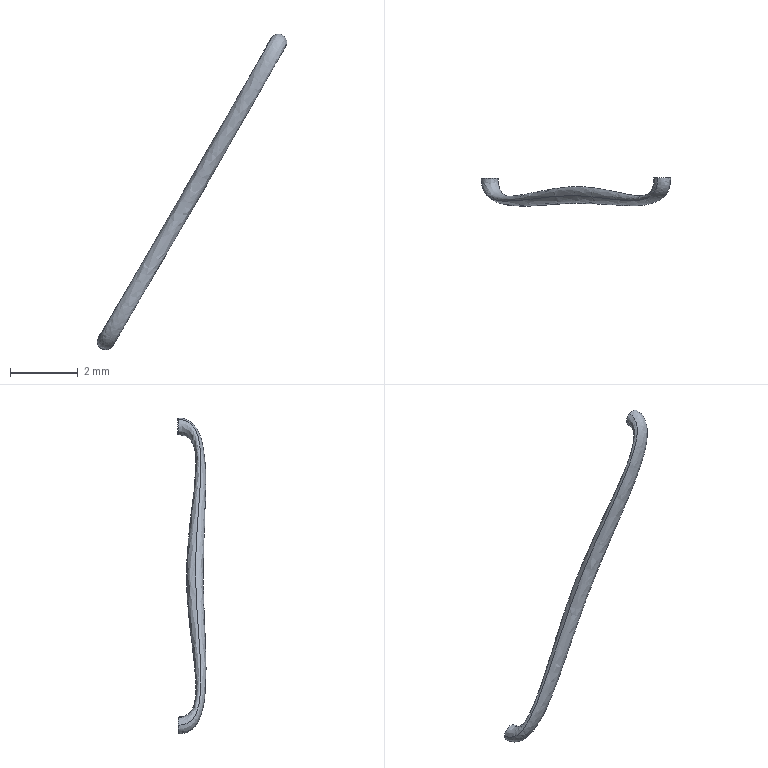Part | SolidWorks | features BaseBody 1 | 1 solid | 4 faces | box 5.609 x 0.83 x 9.35 mm | volume 1.655 mm3 | plane 2 | spline 2
STEP:
#1=CARTESIAN_POINT('',(329.531,392.452,108.323));
#2=VERTEX_POINT('',#1);
#3=CARTESIAN_POINT('',(329.032,392.452,108.347));
#4=VERTEX_POINT('',#3);
#5=CARTESIAN_POINT('',(329.531,392.452,108.323));
#6=CARTESIAN_POINT('',(329.531,392.452,108.316));
#7=CARTESIAN_POINT('',(329.53,392.452,108.303));
#8=CARTESIAN_POINT('',(329.526,392.452,108.283));
#9=CARTESIAN_POINT('',(329.521,392.452,108.263));
#10=CARTESIAN_POINT('',(329.5,392.452,108.201));
#11=CARTESIAN_POINT('',(329.445,392.452,108.134));
#12=CARTESIAN_POINT('',(329.351,392.452,108.091));
#13=CARTESIAN_POINT('',(329.263,392.452,108.08));
#14=CARTESIAN_POINT('',(329.17,392.452,108.104));
#15=CARTESIAN_POINT('',(329.092,392.452,108.163));
#16=CARTESIAN_POINT('',(329.041,392.452,108.246));
#17=CARTESIAN_POINT('',(329.03,392.452,108.314));
#18=CARTESIAN_POINT('',(329.032,392.452,108.347));
#19=B_SPLINE_CURVE_WITH_KNOTS('',3,(#5,#6,#7,#8,#9,#10,#11,#12,#13,#14,#15,#16,#17,#18),.UNSPECIFIED.,.F.,.F.,(4,1,1,1,1,1,1,1,1,1,1,4),(0.,0.025,0.05,0.075,0.1,0.3,0.4,0.5,0.625,0.75,0.875,1.),.UNSPECIFIED.);
#20=EDGE_CURVE('',#2,#4,#19,.T.);
#21=ORIENTED_EDGE('',*,*,#20,.T.);
#22=CARTESIAN_POINT('',(329.032,392.452,108.347));
#23=CARTESIAN_POINT('',(329.034,392.452,108.381));
#24=CARTESIAN_POINT('',(329.051,392.452,108.447));
#25=CARTESIAN_POINT('',(329.11,392.452,108.525));
#26=CARTESIAN_POINT('',(329.192,392.452,108.576));
#27=CARTESIAN_POINT('',(329.287,392.452,108.591));
#28=CARTESIAN_POINT('',(329.374,392.452,108.572));
#29=CARTESIAN_POINT('',(329.464,392.452,108.519));
#30=CARTESIAN_POINT('',(329.512,392.452,108.448));
#31=CARTESIAN_POINT('',(329.527,392.452,108.384));
#32=CARTESIAN_POINT('',(329.53,392.452,108.364));
#33=CARTESIAN_POINT('',(329.532,392.452,108.344));
#34=CARTESIAN_POINT('',(329.532,392.452,108.33));
#35=CARTESIAN_POINT('',(329.531,392.452,108.323));
#36=B_SPLINE_CURVE_WITH_KNOTS('',3,(#22,#23,#24,#25,#26,#27,#28,#29,#30,#31,#32,#33,#34,#35),.UNSPECIFIED.,.F.,.F.,(4,1,1,1,1,1,1,1,1,1,1,4),(0.,0.125,0.25,0.375,0.5,0.6,0.7,0.9,0.925,0.95,0.975,1.),.UNSPECIFIED.);
#37=EDGE_CURVE('',#4,#2,#36,.T.);
#38=ORIENTED_EDGE('',*,*,#37,.T.);
#39=EDGE_LOOP('',(#21,#38));
#40=FACE_OUTER_BOUND('',#39,.T.);
#41=CARTESIAN_POINT('',(329.282,392.452,108.335));
#42=DIRECTION('',(0.0009599,-1.,0.));
#43=DIRECTION('',(0.,0.,-1.));
#44=AXIS2_PLACEMENT_3D('',#41,#42,#43);
#45=PLANE('',#44);
#46=ADVANCED_FACE('',(#40),#45,.F.);
#47=CARTESIAN_POINT('',(334.529,392.457,116.977));
#48=VERTEX_POINT('',#47);
#49=CARTESIAN_POINT('',(334.253,392.457,117.393));
#50=VERTEX_POINT('',#49);
#51=CARTESIAN_POINT('',(334.529,392.457,116.977));
#52=CARTESIAN_POINT('',(334.523,392.457,116.973));
#53=CARTESIAN_POINT('',(334.512,392.457,116.966));
#54=CARTESIAN_POINT('',(334.494,392.457,116.957));
#55=CARTESIAN_POINT('',(334.475,392.457,116.949));
#56=CARTESIAN_POINT('',(334.412,392.457,116.93));
#57=CARTESIAN_POINT('',(334.326,392.457,116.934));
#58=CARTESIAN_POINT('',(334.235,392.457,116.984));
#59=CARTESIAN_POINT('',(334.174,392.457,117.05));
#60=CARTESIAN_POINT('',(334.139,392.457,117.138));
#61=CARTESIAN_POINT('',(334.14,392.457,117.236));
#62=CARTESIAN_POINT('',(334.177,392.457,117.326));
#63=CARTESIAN_POINT('',(334.225,392.457,117.375));
#64=CARTESIAN_POINT('',(334.253,392.457,117.393));
#65=B_SPLINE_CURVE_WITH_KNOTS('',3,(#51,#52,#53,#54,#55,#56,#57,#58,#59,#60,#61,#62,#63,#64),.UNSPECIFIED.,.F.,.F.,(4,1,1,1,1,1,1,1,1,1,1,4),(0.,0.025,0.05,0.075,0.1,0.3,0.4,0.5,0.625,0.75,0.875,1.),.UNSPECIFIED.);
#66=EDGE_CURVE('',#48,#50,#65,.T.);
#67=ORIENTED_EDGE('',*,*,#66,.T.);
#68=CARTESIAN_POINT('',(334.253,392.457,117.393));
#69=CARTESIAN_POINT('',(334.281,392.457,117.412));
#70=CARTESIAN_POINT('',(334.345,392.457,117.437));
#71=CARTESIAN_POINT('',(334.442,392.457,117.436));
#72=CARTESIAN_POINT('',(334.532,392.457,117.399));
#73=CARTESIAN_POINT('',(334.6,392.457,117.332));
#74=CARTESIAN_POINT('',(334.637,392.457,117.251));
#75=CARTESIAN_POINT('',(334.647,392.457,117.147));
#76=CARTESIAN_POINT('',(334.618,392.457,117.066));
#77=CARTESIAN_POINT('',(334.575,392.457,117.016));
#78=CARTESIAN_POINT('',(334.561,392.457,117.002));
#79=CARTESIAN_POINT('',(334.546,392.457,116.988));
#80=CARTESIAN_POINT('',(334.535,392.457,116.98));
#81=CARTESIAN_POINT('',(334.529,392.457,116.977));
#82=B_SPLINE_CURVE_WITH_KNOTS('',3,(#68,#69,#70,#71,#72,#73,#74,#75,#76,#77,#78,#79,#80,#81),.UNSPECIFIED.,.F.,.F.,(4,1,1,1,1,1,1,1,1,1,1,4),(0.,0.125,0.25,0.375,0.5,0.6,0.7,0.9,0.925,0.95,0.975,1.),.UNSPECIFIED.);
#83=EDGE_CURVE('',#50,#48,#82,.T.);
#84=ORIENTED_EDGE('',*,*,#83,.T.);
#85=EDGE_LOOP('',(#67,#84));
#86=FACE_OUTER_BOUND('',#85,.T.);
#87=CARTESIAN_POINT('',(334.391,392.457,117.185));
#88=DIRECTION('',(0.0009599,-1.,0.));
#89=DIRECTION('',(0.,0.,-1.));
#90=AXIS2_PLACEMENT_3D('',#87,#88,#89);
#91=PLANE('',#90);
#92=ADVANCED_FACE('',(#86),#91,.F.);
#93=CARTESIAN_POINT('',(334.253,392.457,117.393));
#94=CARTESIAN_POINT('',(334.254,391.339,117.393));
#95=CARTESIAN_POINT('',(331.637,392.542,112.877));
#96=CARTESIAN_POINT('',(329.033,391.333,108.347));
#97=CARTESIAN_POINT('',(329.032,392.452,108.347));
#98=B_SPLINE_CURVE_WITH_KNOTS('',3,(#93,#94,#95,#96,#97),.UNSPECIFIED.,.F.,.F.,(4,1,4),(0.,0.5,1.),.UNSPECIFIED.);
#99=EDGE_CURVE('',#50,#4,#98,.T.);
#100=ORIENTED_EDGE('',*,*,#99,.T.);
#101=ORIENTED_EDGE('',*,*,#20,.F.);
#102=CARTESIAN_POINT('',(329.531,392.452,108.323));
#103=CARTESIAN_POINT('',(329.532,391.384,108.323));
#104=CARTESIAN_POINT('',(332.113,392.554,112.598));
#105=CARTESIAN_POINT('',(334.53,391.388,116.977));
#106=CARTESIAN_POINT('',(334.529,392.457,116.977));
#107=B_SPLINE_CURVE_WITH_KNOTS('',3,(#102,#103,#104,#105,#106),.UNSPECIFIED.,.F.,.F.,(4,1,4),(0.,0.5,1.),.UNSPECIFIED.);
#108=EDGE_CURVE('',#2,#48,#107,.T.);
#109=ORIENTED_EDGE('',*,*,#108,.T.);
#110=ORIENTED_EDGE('',*,*,#83,.F.);
#111=EDGE_LOOP('',(#100,#101,#109,#110));
#112=FACE_OUTER_BOUND('',#111,.T.);
#113=CARTESIAN_POINT('',(334.512,392.561,116.962));
#114=CARTESIAN_POINT('',(334.591,391.356,117.104));
#115=CARTESIAN_POINT('',(332.117,392.619,112.588));
#116=CARTESIAN_POINT('',(329.445,391.348,108.194));
#117=CARTESIAN_POINT('',(329.536,392.566,108.346));
#118=CARTESIAN_POINT('',(334.517,392.561,116.965));
#119=CARTESIAN_POINT('',(334.596,391.354,117.107));
#120=CARTESIAN_POINT('',(332.115,392.61,112.589));
#121=CARTESIAN_POINT('',(329.445,391.346,108.189));
#122=CARTESIAN_POINT('',(329.536,392.566,108.341));
#123=CARTESIAN_POINT('',(334.527,392.561,116.971));
#124=CARTESIAN_POINT('',(334.607,391.351,117.113));
#125=CARTESIAN_POINT('',(332.112,392.59,112.591));
#126=CARTESIAN_POINT('',(329.445,391.343,108.176));
#127=CARTESIAN_POINT('',(329.536,392.567,108.329));
#128=CARTESIAN_POINT('',(334.542,392.562,116.982));
#129=CARTESIAN_POINT('',(334.623,391.345,117.125));
#130=CARTESIAN_POINT('',(332.105,392.557,112.594));
#131=CARTESIAN_POINT('',(329.443,391.337,108.157));
#132=CARTESIAN_POINT('',(329.534,392.567,108.31));
#133=CARTESIAN_POINT('',(334.558,392.563,116.995));
#134=CARTESIAN_POINT('',(334.639,391.339,117.138));
#135=CARTESIAN_POINT('',(332.097,392.523,112.599));
#136=CARTESIAN_POINT('',(329.44,391.332,108.136));
#137=CARTESIAN_POINT('',(329.531,392.568,108.29));
#138=CARTESIAN_POINT('',(334.572,392.563,117.009));
#139=CARTESIAN_POINT('',(334.654,391.333,117.153));
#140=CARTESIAN_POINT('',(332.087,392.489,112.605));
#141=CARTESIAN_POINT('',(329.435,391.326,108.116));
#142=CARTESIAN_POINT('',(329.526,392.569,108.271));
#143=CARTESIAN_POINT('',(334.614,392.565,117.059));
#144=CARTESIAN_POINT('',(334.699,391.313,117.204));
#145=CARTESIAN_POINT('',(332.05,392.381,112.626));
#146=CARTESIAN_POINT('',(329.415,391.306,108.051));
#147=CARTESIAN_POINT('',(329.505,392.571,108.209));
#148=CARTESIAN_POINT('',(334.643,392.568,117.141));
#149=CARTESIAN_POINT('',(334.731,391.287,117.286));
#150=CARTESIAN_POINT('',(331.979,392.262,112.667));
#151=CARTESIAN_POINT('',(329.36,391.279,107.98));
#152=CARTESIAN_POINT('',(329.449,392.574,108.142));
#153=CARTESIAN_POINT('',(334.633,392.57,117.244));
#154=CARTESIAN_POINT('',(334.723,391.263,117.391));
#155=CARTESIAN_POINT('',(331.876,392.178,112.727));
#156=CARTESIAN_POINT('',(329.266,391.255,107.933));
#157=CARTESIAN_POINT('',(329.355,392.576,108.099));
#158=CARTESIAN_POINT('',(334.596,392.572,117.325));
#159=CARTESIAN_POINT('',(334.689,391.251,117.473));
#160=CARTESIAN_POINT('',(331.787,392.151,112.779));
#161=CARTESIAN_POINT('',(329.178,391.243,107.921));
#162=CARTESIAN_POINT('',(329.267,392.578,108.088));
#163=CARTESIAN_POINT('',(334.528,392.572,117.393));
#164=CARTESIAN_POINT('',(334.621,391.249,117.541));
#165=CARTESIAN_POINT('',(331.703,392.18,112.828));
#166=CARTESIAN_POINT('',(329.085,391.241,107.944));
#167=CARTESIAN_POINT('',(329.174,392.578,108.113));
#168=CARTESIAN_POINT('',(334.438,392.571,117.429));
#169=CARTESIAN_POINT('',(334.53,391.258,117.578));
#170=CARTESIAN_POINT('',(331.643,392.271,112.864));
#171=CARTESIAN_POINT('',(329.007,391.25,108.003));
#172=CARTESIAN_POINT('',(329.097,392.577,108.171));
#173=CARTESIAN_POINT('',(334.34,392.569,117.431));
#174=CARTESIAN_POINT('',(334.43,391.276,117.579));
#175=CARTESIAN_POINT('',(331.615,392.407,112.881));
#176=CARTESIAN_POINT('',(328.955,391.267,108.088));
#177=CARTESIAN_POINT('',(329.045,392.574,108.254));
#178=CARTESIAN_POINT('',(334.272,392.567,117.403));
#179=CARTESIAN_POINT('',(334.359,391.293,117.551));
#180=CARTESIAN_POINT('',(331.623,392.532,112.876));
#181=CARTESIAN_POINT('',(328.942,391.284,108.164));
#182=CARTESIAN_POINT('',(329.034,392.572,108.327));
#183=CARTESIAN_POINT('',(334.241,392.566,117.381));
#184=CARTESIAN_POINT('',(334.327,391.303,117.528));
#185=CARTESIAN_POINT('',(331.636,392.6,112.869));
#186=CARTESIAN_POINT('',(328.945,391.294,108.204));
#187=CARTESIAN_POINT('',(329.037,392.571,108.365));
#188=CARTESIAN_POINT('',(334.237,392.565,117.378));
#189=CARTESIAN_POINT('',(334.322,391.305,117.525));
#190=CARTESIAN_POINT('',(331.638,392.608,112.868));
#191=CARTESIAN_POINT('',(328.946,391.295,108.209));
#192=CARTESIAN_POINT('',(329.038,392.571,108.37));
#193=B_SPLINE_SURFACE_WITH_KNOTS('',3,3,((#113,#114,#115,#116,#117),(#118,#119,#120,#121,#122),(#123,#124,#125,#126,#127),(#128,#129,#130,#131,#132),(#133,#134,#135,#136,#137),(#138,#139,#140,#141,#142),(#143,#144,#145,#146,#147),(#148,#149,#150,#151,#152),(#153,#154,#155,#156,#157),(#158,#159,#160,#161,#162),(#163,#164,#165,#166,#167),(#168,#169,#170,#171,#172),(#173,#174,#175,#176,#177),(#178,#179,#180,#181,#182),(#183,#184,#185,#186,#187),(#188,#189,#190,#191,#192)),.UNSPECIFIED.,.F.,.F.,.F.,(4,1,1,1,1,1,1,1,1,1,1,1,1,4),(4,1,4),(-0.009538,0.,0.0125,0.025,0.0375,0.05,0.15,0.2,0.25,0.3125,0.375,0.4375,0.5,0.5095),(-0.01553,0.5,1.017),.UNSPECIFIED.);
#194=ADVANCED_FACE('',(#112),#193,.T.);
#195=ORIENTED_EDGE('',*,*,#66,.F.);
#196=ORIENTED_EDGE('',*,*,#108,.F.);
#197=ORIENTED_EDGE('',*,*,#37,.F.);
#198=ORIENTED_EDGE('',*,*,#99,.F.);
#199=EDGE_LOOP('',(#195,#196,#197,#198));
#200=FACE_OUTER_BOUND('',#199,.T.);
#201=CARTESIAN_POINT('',(334.262,392.566,117.395));
#202=CARTESIAN_POINT('',(334.349,391.297,117.542));
#203=CARTESIAN_POINT('',(331.628,392.555,112.873));
#204=CARTESIAN_POINT('',(328.944,391.287,108.177));
#205=CARTESIAN_POINT('',(329.036,392.572,108.34));
#206=CARTESIAN_POINT('',(334.258,392.566,117.392));
#207=CARTESIAN_POINT('',(334.344,391.298,117.539));
#208=CARTESIAN_POINT('',(331.63,392.564,112.873));
#209=CARTESIAN_POINT('',(328.944,391.289,108.183));
#210=CARTESIAN_POINT('',(329.036,392.572,108.345));
#211=CARTESIAN_POINT('',(334.225,392.565,117.372));
#212=CARTESIAN_POINT('',(334.31,391.308,117.519));
#213=CARTESIAN_POINT('',(331.64,392.631,112.867));
#214=CARTESIAN_POINT('',(328.945,391.298,108.223));
#215=CARTESIAN_POINT('',(329.037,392.571,108.384));
#216=CARTESIAN_POINT('',(334.173,392.563,117.32));
#217=CARTESIAN_POINT('',(334.255,391.328,117.465));
#218=CARTESIAN_POINT('',(331.677,392.757,112.846));
#219=CARTESIAN_POINT('',(328.963,391.318,108.298));
#220=CARTESIAN_POINT('',(329.055,392.569,108.455));
#221=CARTESIAN_POINT('',(334.137,392.56,117.229));
#222=CARTESIAN_POINT('',(334.215,391.357,117.373));
#223=CARTESIAN_POINT('',(331.755,392.895,112.801));
#224=CARTESIAN_POINT('',(329.021,391.347,108.379));
#225=CARTESIAN_POINT('',(329.114,392.565,108.532));
#226=CARTESIAN_POINT('',(334.135,392.557,117.132));
#227=CARTESIAN_POINT('',(334.211,391.382,117.275));
#228=CARTESIAN_POINT('',(331.849,392.99,112.746));
#229=CARTESIAN_POINT('',(329.103,391.372,108.434));
#230=CARTESIAN_POINT('',(329.197,392.563,108.583));
#231=CARTESIAN_POINT('',(334.171,392.556,117.043));
#232=CARTESIAN_POINT('',(334.245,391.398,117.185));
#233=CARTESIAN_POINT('',(331.945,393.025,112.69));
#234=CARTESIAN_POINT('',(329.198,391.388,108.451));
#235=CARTESIAN_POINT('',(329.292,392.561,108.598));
#236=CARTESIAN_POINT('',(334.232,392.556,116.978));
#237=CARTESIAN_POINT('',(334.305,391.402,117.119));
#238=CARTESIAN_POINT('',(332.024,393.002,112.643));
#239=CARTESIAN_POINT('',(329.285,391.393,108.434));
#240=CARTESIAN_POINT('',(329.379,392.561,108.579));
#241=CARTESIAN_POINT('',(334.323,392.556,116.928));
#242=CARTESIAN_POINT('',(334.396,391.398,117.069));
#243=CARTESIAN_POINT('',(332.098,392.921,112.6));
#244=CARTESIAN_POINT('',(329.375,391.389,108.381));
#245=CARTESIAN_POINT('',(329.468,392.561,108.527));
#246=CARTESIAN_POINT('',(334.409,392.558,116.923));
#247=CARTESIAN_POINT('',(334.484,391.384,117.064));
#248=CARTESIAN_POINT('',(332.126,392.803,112.583));
#249=CARTESIAN_POINT('',(329.424,391.375,108.307));
#250=CARTESIAN_POINT('',(329.516,392.563,108.455));
#251=CARTESIAN_POINT('',(334.472,392.56,116.943));
#252=CARTESIAN_POINT('',(334.549,391.368,117.085));
#253=CARTESIAN_POINT('',(332.124,392.695,112.584));
#254=CARTESIAN_POINT('',(329.44,391.36,108.241));
#255=CARTESIAN_POINT('',(329.532,392.565,108.391));
#256=CARTESIAN_POINT('',(334.49,392.56,116.95));
#257=CARTESIAN_POINT('',(334.568,391.362,117.092));
#258=CARTESIAN_POINT('',(332.122,392.662,112.585));
#259=CARTESIAN_POINT('',(329.443,391.354,108.22));
#260=CARTESIAN_POINT('',(329.535,392.565,108.371));
#261=CARTESIAN_POINT('',(334.508,392.561,116.959));
#262=CARTESIAN_POINT('',(334.587,391.357,117.102));
#263=CARTESIAN_POINT('',(332.118,392.628,112.587));
#264=CARTESIAN_POINT('',(329.445,391.349,108.199));
#265=CARTESIAN_POINT('',(329.536,392.566,108.351));
#266=CARTESIAN_POINT('',(334.524,392.561,116.969));
#267=CARTESIAN_POINT('',(334.604,391.352,117.112));
#268=CARTESIAN_POINT('',(332.113,392.595,112.59));
#269=CARTESIAN_POINT('',(329.445,391.344,108.18));
#270=CARTESIAN_POINT('',(329.536,392.567,108.332));
#271=CARTESIAN_POINT('',(334.534,392.562,116.976));
#272=CARTESIAN_POINT('',(334.614,391.348,117.119));
#273=CARTESIAN_POINT('',(332.109,392.574,112.592));
#274=CARTESIAN_POINT('',(329.444,391.34,108.167));
#275=CARTESIAN_POINT('',(329.535,392.567,108.32));
#276=CARTESIAN_POINT('',(334.538,392.562,116.979));
#277=CARTESIAN_POINT('',(334.619,391.347,117.122));
#278=CARTESIAN_POINT('',(332.107,392.566,112.594));
#279=CARTESIAN_POINT('',(329.444,391.339,108.162));
#280=CARTESIAN_POINT('',(329.535,392.567,108.315));
#281=B_SPLINE_SURFACE_WITH_KNOTS('',3,3,((#201,#202,#203,#204,#205),(#206,#207,#208,#209,#210),(#211,#212,#213,#214,#215),(#216,#217,#218,#219,#220),(#221,#222,#223,#224,#225),(#226,#227,#228,#229,#230),(#231,#232,#233,#234,#235),(#236,#237,#238,#239,#240),(#241,#242,#243,#244,#245),(#246,#247,#248,#249,#250),(#251,#252,#253,#254,#255),(#256,#257,#258,#259,#260),(#261,#262,#263,#264,#265),(#266,#267,#268,#269,#270),(#271,#272,#273,#274,#275),(#276,#277,#278,#279,#280)),.UNSPECIFIED.,.F.,.F.,.F.,(4,1,1,1,1,1,1,1,1,1,1,1,1,4),(4,1,4),(0.4905,0.5,0.5625,0.625,0.6875,0.75,0.8,0.85,0.95,0.9625,0.975,0.9875,1.,1.01),(-0.01553,0.5,1.017),.UNSPECIFIED.);
#282=ADVANCED_FACE('',(#200),#281,.T.);
#283=CLOSED_SHELL('',(#46,#92,#194,#282));
#284=MANIFOLD_SOLID_BREP('',#283);
#285=CARTESIAN_POINT('',(0.,0.,0.));
#286=DIRECTION('',(0.,0.,1.));
#287=DIRECTION('',(1.,0.,0.));
#288=AXIS2_PLACEMENT_3D('',#285,#286,#287);
#289=(LENGTH_UNIT()NAMED_UNIT(*)SI_UNIT(.MILLI.,.METRE.));
#290=UNCERTAINTY_MEASURE_WITH_UNIT(LENGTH_MEASURE(0.00001),#289,'','');
#291=(NAMED_UNIT(*)PLANE_ANGLE_UNIT()SI_UNIT($,.RADIAN.));
#292=(NAMED_UNIT(*)SI_UNIT($,.STERADIAN.)SOLID_ANGLE_UNIT());
#293=(GEOMETRIC_REPRESENTATION_CONTEXT(3)GLOBAL_UNCERTAINTY_ASSIGNED_CONTEXT((#290))GLOBAL_UNIT_ASSIGNED_CONTEXT((#289,#291,#292))REPRESENTATION_CONTEXT('',''));
#294=ADVANCED_BREP_SHAPE_REPRESENTATION('',(#284,#288),#293);